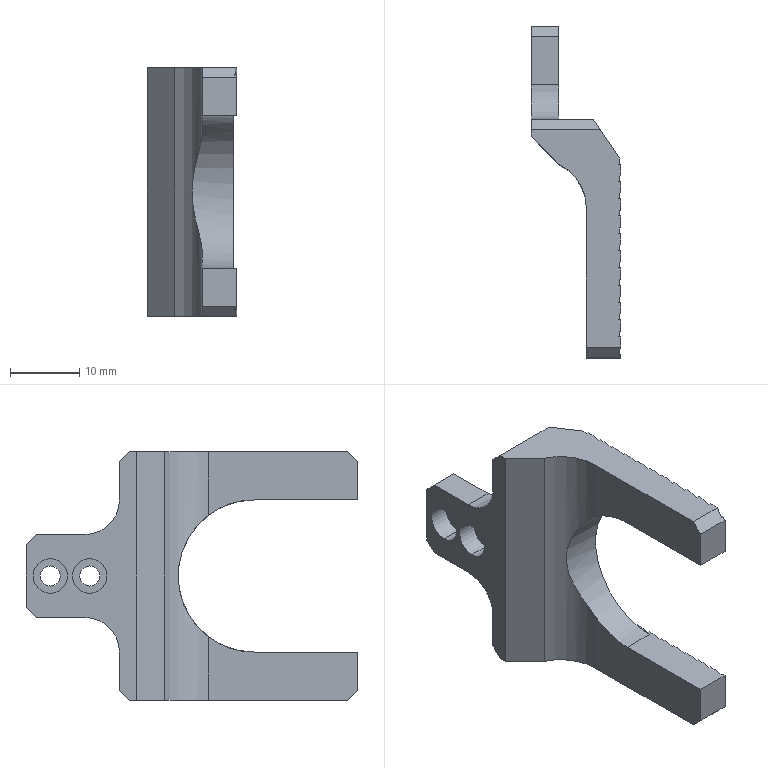Part | STEP file | 0-19 Finger 2 (original) | 1 solid | 109 faces | box 13 x 48 x 36 mm | volume 5429 mm3 | plane 97 | cylinder 12 | commonest cylinder face diameters 2.9 x4 5 x4 10 x2 14 x1 22 x1